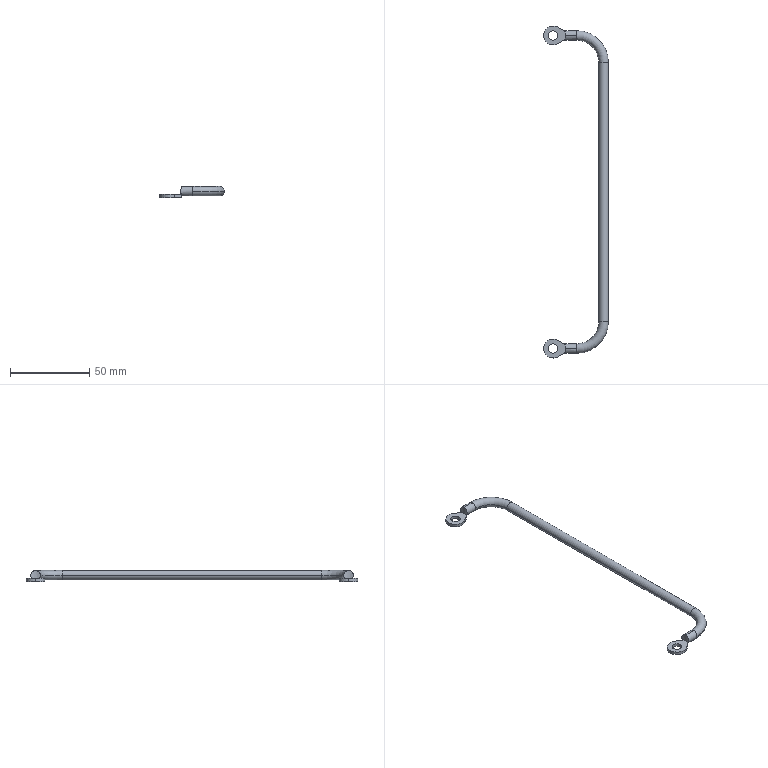Part | SolidWorks | features BaseBody 1 | 1 solid | 30 faces | box 41 x 210 x 7 mm | volume 6943 mm3 | cylinder 16 | plane 10 | torus 4 | commonest cylinder face diameters 6 x10 12 x4 16 x2
STEP:
#1=CARTESIAN_POINT('',(7.681,2.236,-4.));
#2=VERTEX_POINT('',#1);
#3=CARTESIAN_POINT('',(7.681,2.236,-2.));
#4=VERTEX_POINT('',#3);
#5=CARTESIAN_POINT('',(7.681,2.236,-15.078));
#6=DIRECTION('',(0.,0.,1.));
#7=VECTOR('',#6,1000.);
#8=LINE('',#5,#7);
#9=EDGE_CURVE('',#2,#4,#8,.T.);
#10=ORIENTED_EDGE('',*,*,#9,.F.);
#11=CARTESIAN_POINT('',(3.211,5.068,-4.));
#12=VERTEX_POINT('',#11);
#13=CARTESIAN_POINT('',(3.211,5.068,-4.));
#14=DIRECTION('',(-0.8447,0.5352,0.));
#15=VECTOR('',#14,1000.);
#16=LINE('',#13,#15);
#17=EDGE_CURVE('',#2,#12,#16,.T.);
#18=ORIENTED_EDGE('',*,*,#17,.T.);
#19=CARTESIAN_POINT('',(3.211,5.068,-2.));
#20=VERTEX_POINT('',#19);
#21=CARTESIAN_POINT('',(3.211,5.068,-15.078));
#22=DIRECTION('',(0.,0.,1.));
#23=VECTOR('',#22,1000.);
#24=LINE('',#21,#23);
#25=EDGE_CURVE('',#12,#20,#24,.T.);
#26=ORIENTED_EDGE('',*,*,#25,.T.);
#27=CARTESIAN_POINT('',(3.211,5.068,-2.));
#28=DIRECTION('',(0.8447,-0.5352,0.));
#29=VECTOR('',#28,1000.);
#30=LINE('',#27,#29);
#31=EDGE_CURVE('',#20,#4,#30,.T.);
#32=ORIENTED_EDGE('',*,*,#31,.T.);
#33=EDGE_LOOP('',(#10,#18,#26,#32));
#34=FACE_OUTER_BOUND('',#33,.T.);
#35=CARTESIAN_POINT('',(3.211,5.068,-15.078));
#36=DIRECTION('',(-0.5352,-0.8447,0.));
#37=DIRECTION('',(-0.8447,0.5352,0.));
#38=AXIS2_PLACEMENT_3D('',#35,#36,#37);
#39=PLANE('',#38);
#40=ADVANCED_FACE('',(#34),#39,.F.);
#41=CARTESIAN_POINT('',(7.681,-2.236,-2.));
#42=VERTEX_POINT('',#41);
#43=CARTESIAN_POINT('',(7.681,0.,-3.));
#44=VERTEX_POINT('',#43);
#45=CARTESIAN_POINT('',(7.681,0.,0.));
#46=DIRECTION('',(1.,0.,0.));
#47=DIRECTION('',(0.,0.,1.));
#48=AXIS2_PLACEMENT_3D('',#45,#46,#47);
#49=CIRCLE('',#48,3.);
#50=EDGE_CURVE('',#42,#44,#49,.T.);
#51=ORIENTED_EDGE('',*,*,#50,.F.);
#52=CARTESIAN_POINT('',(7.681,-2.236,-4.));
#53=VERTEX_POINT('',#52);
#54=CARTESIAN_POINT('',(7.681,-2.236,-15.078));
#55=DIRECTION('',(0.,0.,1.));
#56=VECTOR('',#55,1000.);
#57=LINE('',#54,#56);
#58=EDGE_CURVE('',#53,#42,#57,.T.);
#59=ORIENTED_EDGE('',*,*,#58,.F.);
#60=CARTESIAN_POINT('',(7.681,2.236,-4.));
#61=DIRECTION('',(0.,1.,0.));
#62=VECTOR('',#61,1000.);
#63=LINE('',#60,#62);
#64=EDGE_CURVE('',#53,#2,#63,.T.);
#65=ORIENTED_EDGE('',*,*,#64,.T.);
#66=ORIENTED_EDGE('',*,*,#9,.T.);
#67=CARTESIAN_POINT('',(7.681,0.,0.));
#68=DIRECTION('',(1.,0.,0.));
#69=DIRECTION('',(0.,0.,1.));
#70=AXIS2_PLACEMENT_3D('',#67,#68,#69);
#71=CIRCLE('',#70,3.);
#72=EDGE_CURVE('',#44,#4,#71,.T.);
#73=ORIENTED_EDGE('',*,*,#72,.F.);
#74=EDGE_LOOP('',(#51,#59,#65,#66,#73));
#75=FACE_OUTER_BOUND('',#74,.T.);
#76=CARTESIAN_POINT('',(7.681,2.236,-15.078));
#77=DIRECTION('',(-1.,0.,0.));
#78=DIRECTION('',(0.,0.,1.));
#79=AXIS2_PLACEMENT_3D('',#76,#77,#78);
#80=PLANE('',#79);
#81=ADVANCED_FACE('',(#75),#80,.F.);
#82=CARTESIAN_POINT('',(3.211,-5.068,-4.));
#83=VERTEX_POINT('',#82);
#84=CARTESIAN_POINT('',(3.211,-5.068,-2.));
#85=VERTEX_POINT('',#84);
#86=CARTESIAN_POINT('',(3.211,-5.068,-15.078));
#87=DIRECTION('',(0.,0.,1.));
#88=VECTOR('',#87,1000.);
#89=LINE('',#86,#88);
#90=EDGE_CURVE('',#83,#85,#89,.T.);
#91=ORIENTED_EDGE('',*,*,#90,.F.);
#92=CARTESIAN_POINT('',(7.681,-2.236,-4.));
#93=DIRECTION('',(0.8447,0.5352,0.));
#94=VECTOR('',#93,1000.);
#95=LINE('',#92,#94);
#96=EDGE_CURVE('',#83,#53,#95,.T.);
#97=ORIENTED_EDGE('',*,*,#96,.T.);
#98=ORIENTED_EDGE('',*,*,#58,.T.);
#99=CARTESIAN_POINT('',(7.681,-2.236,-2.));
#100=DIRECTION('',(-0.8447,-0.5352,0.));
#101=VECTOR('',#100,1000.);
#102=LINE('',#99,#101);
#103=EDGE_CURVE('',#42,#85,#102,.T.);
#104=ORIENTED_EDGE('',*,*,#103,.T.);
#105=EDGE_LOOP('',(#91,#97,#98,#104));
#106=FACE_OUTER_BOUND('',#105,.T.);
#107=CARTESIAN_POINT('',(7.681,-2.236,-15.078));
#108=DIRECTION('',(-0.5352,0.8447,0.));
#109=DIRECTION('',(0.,0.,1.));
#110=AXIS2_PLACEMENT_3D('',#107,#108,#109);
#111=PLANE('',#110);
#112=ADVANCED_FACE('',(#106),#111,.F.);
#113=CARTESIAN_POINT('',(7.681,200.236,-4.));
#114=VERTEX_POINT('',#113);
#115=CARTESIAN_POINT('',(7.681,200.236,-2.));
#116=VERTEX_POINT('',#115);
#117=CARTESIAN_POINT('',(7.681,200.236,-15.078));
#118=DIRECTION('',(0.,0.,1.));
#119=VECTOR('',#118,1000.);
#120=LINE('',#117,#119);
#121=EDGE_CURVE('',#114,#116,#120,.T.);
#122=ORIENTED_EDGE('',*,*,#121,.F.);
#123=CARTESIAN_POINT('',(3.211,203.068,-4.));
#124=VERTEX_POINT('',#123);
#125=CARTESIAN_POINT('',(3.211,203.068,-4.));
#126=DIRECTION('',(-0.8447,0.5352,0.));
#127=VECTOR('',#126,1000.);
#128=LINE('',#125,#127);
#129=EDGE_CURVE('',#114,#124,#128,.T.);
#130=ORIENTED_EDGE('',*,*,#129,.T.);
#131=CARTESIAN_POINT('',(3.211,203.068,-2.));
#132=VERTEX_POINT('',#131);
#133=CARTESIAN_POINT('',(3.211,203.068,-15.078));
#134=DIRECTION('',(0.,0.,1.));
#135=VECTOR('',#134,1000.);
#136=LINE('',#133,#135);
#137=EDGE_CURVE('',#124,#132,#136,.T.);
#138=ORIENTED_EDGE('',*,*,#137,.T.);
#139=CARTESIAN_POINT('',(3.211,203.068,-2.));
#140=DIRECTION('',(0.8447,-0.5352,0.));
#141=VECTOR('',#140,1000.);
#142=LINE('',#139,#141);
#143=EDGE_CURVE('',#132,#116,#142,.T.);
#144=ORIENTED_EDGE('',*,*,#143,.T.);
#145=EDGE_LOOP('',(#122,#130,#138,#144));
#146=FACE_OUTER_BOUND('',#145,.T.);
#147=CARTESIAN_POINT('',(3.211,203.068,-15.078));
#148=DIRECTION('',(-0.5352,-0.8447,0.));
#149=DIRECTION('',(-0.8447,0.5352,0.));
#150=AXIS2_PLACEMENT_3D('',#147,#148,#149);
#151=PLANE('',#150);
#152=ADVANCED_FACE('',(#146),#151,.F.);
#153=CARTESIAN_POINT('',(7.681,195.764,-2.));
#154=VERTEX_POINT('',#153);
#155=CARTESIAN_POINT('',(7.681,198.,-3.));
#156=VERTEX_POINT('',#155);
#157=CARTESIAN_POINT('',(7.681,198.,0.));
#158=DIRECTION('',(1.,0.,0.));
#159=DIRECTION('',(0.,-1.,0.));
#160=AXIS2_PLACEMENT_3D('',#157,#158,#159);
#161=CIRCLE('',#160,3.);
#162=EDGE_CURVE('',#154,#156,#161,.T.);
#163=ORIENTED_EDGE('',*,*,#162,.F.);
#164=CARTESIAN_POINT('',(7.681,195.764,-4.));
#165=VERTEX_POINT('',#164);
#166=CARTESIAN_POINT('',(7.681,195.764,-15.078));
#167=DIRECTION('',(0.,0.,1.));
#168=VECTOR('',#167,1000.);
#169=LINE('',#166,#168);
#170=EDGE_CURVE('',#165,#154,#169,.T.);
#171=ORIENTED_EDGE('',*,*,#170,.F.);
#172=CARTESIAN_POINT('',(7.681,200.236,-4.));
#173=DIRECTION('',(0.,1.,0.));
#174=VECTOR('',#173,1000.);
#175=LINE('',#172,#174);
#176=EDGE_CURVE('',#165,#114,#175,.T.);
#177=ORIENTED_EDGE('',*,*,#176,.T.);
#178=ORIENTED_EDGE('',*,*,#121,.T.);
#179=CARTESIAN_POINT('',(7.681,198.,0.));
#180=DIRECTION('',(1.,0.,0.));
#181=DIRECTION('',(0.,-1.,0.));
#182=AXIS2_PLACEMENT_3D('',#179,#180,#181);
#183=CIRCLE('',#182,3.);
#184=EDGE_CURVE('',#156,#116,#183,.T.);
#185=ORIENTED_EDGE('',*,*,#184,.F.);
#186=EDGE_LOOP('',(#163,#171,#177,#178,#185));
#187=FACE_OUTER_BOUND('',#186,.T.);
#188=CARTESIAN_POINT('',(7.681,200.236,-15.078));
#189=DIRECTION('',(-1.,0.,0.));
#190=DIRECTION('',(0.,0.,1.));
#191=AXIS2_PLACEMENT_3D('',#188,#189,#190);
#192=PLANE('',#191);
#193=ADVANCED_FACE('',(#187),#192,.F.);
#194=CARTESIAN_POINT('',(3.211,192.932,-4.));
#195=VERTEX_POINT('',#194);
#196=CARTESIAN_POINT('',(3.211,192.932,-2.));
#197=VERTEX_POINT('',#196);
#198=CARTESIAN_POINT('',(3.211,192.932,-15.078));
#199=DIRECTION('',(0.,0.,1.));
#200=VECTOR('',#199,1000.);
#201=LINE('',#198,#200);
#202=EDGE_CURVE('',#195,#197,#201,.T.);
#203=ORIENTED_EDGE('',*,*,#202,.F.);
#204=CARTESIAN_POINT('',(3.211,192.932,-4.));
#205=DIRECTION('',(0.8447,0.5352,0.));
#206=VECTOR('',#205,1000.);
#207=LINE('',#204,#206);
#208=EDGE_CURVE('',#195,#165,#207,.T.);
#209=ORIENTED_EDGE('',*,*,#208,.T.);
#210=ORIENTED_EDGE('',*,*,#170,.T.);
#211=CARTESIAN_POINT('',(3.211,192.932,-2.));
#212=DIRECTION('',(-0.8447,-0.5352,0.));
#213=VECTOR('',#212,1000.);
#214=LINE('',#211,#213);
#215=EDGE_CURVE('',#154,#197,#214,.T.);
#216=ORIENTED_EDGE('',*,*,#215,.T.);
#217=EDGE_LOOP('',(#203,#209,#210,#216));
#218=FACE_OUTER_BOUND('',#217,.T.);
#219=CARTESIAN_POINT('',(3.211,192.932,-15.078));
#220=DIRECTION('',(-0.5352,0.8447,0.));
#221=DIRECTION('',(0.,0.,1.));
#222=AXIS2_PLACEMENT_3D('',#219,#220,#221);
#223=PLANE('',#222);
#224=ADVANCED_FACE('',(#218),#223,.F.);
#225=CARTESIAN_POINT('',(0.,0.,-2.));
#226=DIRECTION('',(0.,0.,1.));
#227=DIRECTION('',(1.,0.,0.));
#228=AXIS2_PLACEMENT_3D('',#225,#226,#227);
#229=CIRCLE('',#228,8.);
#230=EDGE_CURVE('',#42,#4,#229,.T.);
#231=ORIENTED_EDGE('',*,*,#230,.F.);
#232=CARTESIAN_POINT('',(8.,0.,3.));
#233=VERTEX_POINT('',#232);
#234=CARTESIAN_POINT('',(8.,0.,3.));
#235=CARTESIAN_POINT('',(8.,-0.1411,3.));
#236=CARTESIAN_POINT('',(7.996,-0.284,2.99));
#237=CARTESIAN_POINT('',(7.985,-0.499,2.959));
#238=CARTESIAN_POINT('',(7.98,-0.5708,2.946));
#239=CARTESIAN_POINT('',(7.971,-0.6783,2.923));
#240=CARTESIAN_POINT('',(7.967,-0.732,2.91));
#241=CARTESIAN_POINT('',(7.96,-0.7945,2.893));
#242=CARTESIAN_POINT('',(7.958,-0.8212,2.885));
#243=CARTESIAN_POINT('',(7.956,-0.839,2.88));
#244=CARTESIAN_POINT('',(7.955,-0.8491,2.877));
#245=CARTESIAN_POINT('',(7.941,-0.9804,2.838));
#246=CARTESIAN_POINT('',(7.924,-1.109,2.791));
#247=CARTESIAN_POINT('',(7.893,-1.305,2.702));
#248=CARTESIAN_POINT('',(7.882,-1.371,2.669));
#249=CARTESIAN_POINT('',(7.864,-1.47,2.615));
#250=CARTESIAN_POINT('',(7.854,-1.52,2.587));
#251=CARTESIAN_POINT('',(7.843,-1.578,2.551));
#252=CARTESIAN_POINT('',(7.837,-1.607,2.533));
#253=CARTESIAN_POINT('',(7.834,-1.62,2.525));
#254=CARTESIAN_POINT('',(7.833,-1.628,2.52));
#255=CARTESIAN_POINT('',(7.832,-1.633,2.516));
#256=CARTESIAN_POINT('',(7.82,-1.687,2.481));
#257=CARTESIAN_POINT('',(7.808,-1.741,2.444));
#258=CARTESIAN_POINT('',(7.789,-1.827,2.38));
#259=CARTESIAN_POINT('',(7.782,-1.856,2.357));
#260=CARTESIAN_POINT('',(7.771,-1.901,2.321));
#261=CARTESIAN_POINT('',(7.765,-1.924,2.302));
#262=CARTESIAN_POINT('',(7.76,-1.947,2.283));
#263=CARTESIAN_POINT('',(7.756,-1.962,2.27));
#264=CARTESIAN_POINT('',(7.753,-1.971,2.262));
#265=CARTESIAN_POINT('',(7.738,-2.031,2.209));
#266=CARTESIAN_POINT('',(7.717,-2.109,2.136));
#267=CARTESIAN_POINT('',(7.693,-2.195,2.046));
#268=CARTESIAN_POINT('',(7.681,-2.237,1.999));
#269=CARTESIAN_POINT('',(7.676,-2.254,1.979));
#270=CARTESIAN_POINT('',(7.672,-2.266,1.966));
#271=CARTESIAN_POINT('',(7.671,-2.271,1.96));
#272=CARTESIAN_POINT('',(7.636,-2.386,1.826));
#273=CARTESIAN_POINT('',(7.608,-2.476,1.7));
#274=CARTESIAN_POINT('',(7.57,-2.589,1.518));
#275=CARTESIAN_POINT('',(7.558,-2.622,1.459));
#276=CARTESIAN_POINT('',(7.542,-2.668,1.371));
#277=CARTESIAN_POINT('',(7.534,-2.69,1.329));
#278=CARTESIAN_POINT('',(7.526,-2.713,1.28));
#279=CARTESIAN_POINT('',(7.522,-2.723,1.259));
#280=CARTESIAN_POINT('',(7.52,-2.729,1.245));
#281=CARTESIAN_POINT('',(7.519,-2.732,1.24));
#282=CARTESIAN_POINT('',(7.495,-2.799,1.091));
#283=CARTESIAN_POINT('',(7.476,-2.849,0.9501));
#284=CARTESIAN_POINT('',(7.453,-2.908,0.7416));
#285=CARTESIAN_POINT('',(7.446,-2.924,0.6726));
#286=CARTESIAN_POINT('',(7.438,-2.946,0.5701));
#287=CARTESIAN_POINT('',(7.434,-2.955,0.5191));
#288=CARTESIAN_POINT('',(7.431,-2.963,0.4685));
#289=CARTESIAN_POINT('',(7.429,-2.968,0.435));
#290=CARTESIAN_POINT('',(7.428,-2.971,0.4194));
#291=CARTESIAN_POINT('',(7.419,-2.992,0.2582));
#292=CARTESIAN_POINT('',(7.416,-3.001,0.1133));
#293=CARTESIAN_POINT('',(7.417,-2.999,-0.1042));
#294=CARTESIAN_POINT('',(7.418,-2.996,-0.1767));
#295=CARTESIAN_POINT('',(7.422,-2.987,-0.2852));
#296=CARTESIAN_POINT('',(7.424,-2.981,-0.3393));
#297=CARTESIAN_POINT('',(7.427,-2.974,-0.3934));
#298=CARTESIAN_POINT('',(7.429,-2.969,-0.4293));
#299=CARTESIAN_POINT('',(7.43,-2.966,-0.4488));
#300=CARTESIAN_POINT('',(7.439,-2.943,-0.5972));
#301=CARTESIAN_POINT('',(7.451,-2.913,-0.733));
#302=CARTESIAN_POINT('',(7.475,-2.85,-0.94));
#303=CARTESIAN_POINT('',(7.484,-2.826,-1.009));
#304=CARTESIAN_POINT('',(7.499,-2.786,-1.114));
#305=CARTESIAN_POINT('',(7.507,-2.764,-1.166));
#306=CARTESIAN_POINT('',(7.517,-2.737,-1.228));
#307=CARTESIAN_POINT('',(7.522,-2.723,-1.258));
#308=CARTESIAN_POINT('',(7.524,-2.717,-1.271));
#309=CARTESIAN_POINT('',(7.526,-2.713,-1.28));
#310=CARTESIAN_POINT('',(7.527,-2.71,-1.286));
#311=CARTESIAN_POINT('',(7.56,-2.618,-1.48));
#312=CARTESIAN_POINT('',(7.611,-2.476,-1.732));
#313=CARTESIAN_POINT('',(7.681,-2.236,-2.));
#314=B_SPLINE_CURVE_WITH_KNOTS('',3,(#234,#235,#236,#237,#238,#239,#240,#241,#242,#243,#244,#245,#246,#247,#248,#249,#250,#251,#252,#253,#254,#255,#256,#257,#258,#259,#260,#261,#262,#263,#264,#265,#266,#267,#268,#269,#270,#271,#272,#273,#274,#275,#276,#277,#278,#279,#280,#281,#282,#283,#284,#285,#286,#287,#288,#289,#290,#291,#292,#293,#294,#295,#296,#297,#298,#299,#300,#301,#302,#303,#304,#305,#306,#307,#308,#309,#310,#311,#312,#313),.UNSPECIFIED.,.F.,.F.,(4,2,2,1,1,2,2,2,2,1,1,1,2,2,2,2,1,2,2,1,1,1,2,2,2,2,1,1,2,2,2,2,1,2,2,2,2,1,2,2,2,2,1,1,1,2,2,4),(0.,0.0625,0.09375,0.1094,0.1172,0.1211,0.125,0.1875,0.2187,0.2344,0.2422,0.2461,0.248,0.25,0.2812,0.2969,0.3047,0.3086,0.3125,0.3437,0.3594,0.3672,0.3711,0.375,0.4375,0.4687,0.4844,0.4922,0.4961,0.5,0.5625,0.5937,0.6094,0.6172,0.625,0.6875,0.7187,0.7344,0.7422,0.75,0.8125,0.8437,0.8594,0.8672,0.8711,0.873,0.875,1.),.UNSPECIFIED.);
#315=EDGE_CURVE('',#233,#42,#314,.T.);
#316=ORIENTED_EDGE('',*,*,#315,.F.);
#317=CARTESIAN_POINT('',(7.681,2.236,-2.));
#318=CARTESIAN_POINT('',(7.646,2.356,-1.866));
#319=CARTESIAN_POINT('',(7.616,2.452,-1.735));
#320=CARTESIAN_POINT('',(7.577,2.567,-1.554));
#321=CARTESIAN_POINT('',(7.566,2.601,-1.497));
#322=CARTESIAN_POINT('',(7.55,2.646,-1.415));
#323=CARTESIAN_POINT('',(7.543,2.667,-1.375));
#324=CARTESIAN_POINT('',(7.535,2.689,-1.331));
#325=CARTESIAN_POINT('',(7.531,2.699,-1.309));
#326=CARTESIAN_POINT('',(7.529,2.704,-1.3));
#327=CARTESIAN_POINT('',(7.528,2.706,-1.294));
#328=CARTESIAN_POINT('',(7.528,2.707,-1.293));
#329=CARTESIAN_POINT('',(7.503,2.776,-1.149));
#330=CARTESIAN_POINT('',(7.483,2.829,-1.009));
#331=CARTESIAN_POINT('',(7.459,2.892,-0.8019));
#332=CARTESIAN_POINT('',(7.452,2.91,-0.7335));
#333=CARTESIAN_POINT('',(7.443,2.933,-0.632));
#334=CARTESIAN_POINT('',(7.439,2.943,-0.5815));
#335=CARTESIAN_POINT('',(7.435,2.953,-0.5315));
#336=CARTESIAN_POINT('',(7.433,2.958,-0.4983));
#337=CARTESIAN_POINT('',(7.432,2.961,-0.4832));
#338=CARTESIAN_POINT('',(7.422,2.986,-0.3218));
#339=CARTESIAN_POINT('',(7.417,2.998,-0.1769));
#340=CARTESIAN_POINT('',(7.416,3.001,0.04039));
#341=CARTESIAN_POINT('',(7.417,2.999,0.1128));
#342=CARTESIAN_POINT('',(7.419,2.992,0.2211));
#343=CARTESIAN_POINT('',(7.421,2.988,0.2752));
#344=CARTESIAN_POINT('',(7.423,2.982,0.3292));
#345=CARTESIAN_POINT('',(7.425,2.978,0.3651));
#346=CARTESIAN_POINT('',(7.426,2.975,0.3842));
#347=CARTESIAN_POINT('',(7.434,2.955,0.5349));
#348=CARTESIAN_POINT('',(7.445,2.927,0.6725));
#349=CARTESIAN_POINT('',(7.468,2.868,0.8818));
#350=CARTESIAN_POINT('',(7.477,2.846,0.9521));
#351=CARTESIAN_POINT('',(7.491,2.808,1.058));
#352=CARTESIAN_POINT('',(7.499,2.787,1.111));
#353=CARTESIAN_POINT('',(7.508,2.762,1.172));
#354=CARTESIAN_POINT('',(7.513,2.748,1.203));
#355=CARTESIAN_POINT('',(7.515,2.742,1.217));
#356=CARTESIAN_POINT('',(7.517,2.738,1.225));
#357=CARTESIAN_POINT('',(7.518,2.736,1.231));
#358=CARTESIAN_POINT('',(7.535,2.689,1.334));
#359=CARTESIAN_POINT('',(7.555,2.632,1.447));
#360=CARTESIAN_POINT('',(7.593,2.52,1.63));
#361=CARTESIAN_POINT('',(7.607,2.478,1.693));
#362=CARTESIAN_POINT('',(7.629,2.408,1.79));
#363=CARTESIAN_POINT('',(7.641,2.371,1.838));
#364=CARTESIAN_POINT('',(7.655,2.325,1.896));
#365=CARTESIAN_POINT('',(7.661,2.304,1.921));
#366=CARTESIAN_POINT('',(7.665,2.29,1.938));
#367=CARTESIAN_POINT('',(7.668,2.282,1.948));
#368=CARTESIAN_POINT('',(7.697,2.183,2.062));
#369=CARTESIAN_POINT('',(7.725,2.082,2.164));
#370=CARTESIAN_POINT('',(7.766,1.923,2.304));
#371=CARTESIAN_POINT('',(7.779,1.868,2.349));
#372=CARTESIAN_POINT('',(7.799,1.782,2.413));
#373=CARTESIAN_POINT('',(7.809,1.739,2.445));
#374=CARTESIAN_POINT('',(7.818,1.695,2.475));
#375=CARTESIAN_POINT('',(7.825,1.665,2.495));
#376=CARTESIAN_POINT('',(7.828,1.652,2.504));
#377=CARTESIAN_POINT('',(7.859,1.503,2.601));
#378=CARTESIAN_POINT('',(7.883,1.37,2.673));
#379=CARTESIAN_POINT('',(7.914,1.174,2.762));
#380=CARTESIAN_POINT('',(7.923,1.109,2.788));
#381=CARTESIAN_POINT('',(7.936,1.013,2.824));
#382=CARTESIAN_POINT('',(7.942,0.9659,2.841));
#383=CARTESIAN_POINT('',(7.948,0.9112,2.858));
#384=CARTESIAN_POINT('',(7.951,0.8879,2.866));
#385=CARTESIAN_POINT('',(7.952,0.8724,2.87));
#386=CARTESIAN_POINT('',(7.953,0.8659,2.872));
#387=CARTESIAN_POINT('',(7.985,0.5721,2.96));
#388=CARTESIAN_POINT('',(8.,0.2822,3.));
#389=CARTESIAN_POINT('',(8.,0.,3.));
#390=B_SPLINE_CURVE_WITH_KNOTS('',3,(#317,#318,#319,#320,#321,#322,#323,#324,#325,#326,#327,#328,#329,#330,#331,#332,#333,#334,#335,#336,#337,#338,#339,#340,#341,#342,#343,#344,#345,#346,#347,#348,#349,#350,#351,#352,#353,#354,#355,#356,#357,#358,#359,#360,#361,#362,#363,#364,#365,#366,#367,#368,#369,#370,#371,#372,#373,#374,#375,#376,#377,#378,#379,#380,#381,#382,#383,#384,#385,#386,#387,#388,#389),.UNSPECIFIED.,.F.,.F.,(4,2,2,1,1,1,2,2,2,2,1,2,2,2,2,1,2,2,2,2,1,1,1,2,2,2,2,1,1,2,2,2,2,1,2,2,2,2,1,1,2,2,4),(0.,0.0625,0.09375,0.1094,0.1172,0.1211,0.123,0.125,0.1875,0.2188,0.2344,0.2422,0.25,0.3125,0.3438,0.3594,0.3672,0.375,0.4375,0.4688,0.4844,0.4922,0.4961,0.498,0.5,0.5625,0.5938,0.6094,0.6172,0.6211,0.625,0.6875,0.7188,0.7344,0.7422,0.75,0.8125,0.8438,0.8594,0.8672,0.8711,0.875,1.),.UNSPECIFIED.);
#391=EDGE_CURVE('',#4,#233,#390,.T.);
#392=ORIENTED_EDGE('',*,*,#391,.F.);
#393=EDGE_LOOP('',(#231,#316,#392));
#394=FACE_OUTER_BOUND('',#393,.T.);
#395=CARTESIAN_POINT('',(0.,0.,13.));
#396=DIRECTION('',(0.,0.,-1.));
#397=DIRECTION('',(-1.,0.,0.));
#398=AXIS2_PLACEMENT_3D('',#395,#396,#397);
#399=CYLINDRICAL_SURFACE('',#398,8.);
#400=ADVANCED_FACE('',(#394),#399,.F.);
#401=CARTESIAN_POINT('',(0.,198.,-2.));
#402=DIRECTION('',(0.,0.,1.));
#403=DIRECTION('',(1.,0.,0.));
#404=AXIS2_PLACEMENT_3D('',#401,#402,#403);
#405=CIRCLE('',#404,8.);
#406=EDGE_CURVE('',#154,#116,#405,.T.);
#407=ORIENTED_EDGE('',*,*,#406,.F.);
#408=CARTESIAN_POINT('',(8.,198.,3.));
#409=VERTEX_POINT('',#408);
#410=CARTESIAN_POINT('',(8.,198.,3.));
#411=CARTESIAN_POINT('',(8.,197.859,3.));
#412=CARTESIAN_POINT('',(7.996,197.716,2.99));
#413=CARTESIAN_POINT('',(7.985,197.501,2.959));
#414=CARTESIAN_POINT('',(7.98,197.429,2.946));
#415=CARTESIAN_POINT('',(7.971,197.322,2.923));
#416=CARTESIAN_POINT('',(7.967,197.268,2.91));
#417=CARTESIAN_POINT('',(7.96,197.206,2.893));
#418=CARTESIAN_POINT('',(7.958,197.179,2.885));
#419=CARTESIAN_POINT('',(7.956,197.161,2.88));
#420=CARTESIAN_POINT('',(7.955,197.151,2.877));
#421=CARTESIAN_POINT('',(7.941,197.02,2.838));
#422=CARTESIAN_POINT('',(7.924,196.891,2.791));
#423=CARTESIAN_POINT('',(7.893,196.695,2.702));
#424=CARTESIAN_POINT('',(7.882,196.629,2.669));
#425=CARTESIAN_POINT('',(7.864,196.53,2.615));
#426=CARTESIAN_POINT('',(7.854,196.48,2.587));
#427=CARTESIAN_POINT('',(7.843,196.422,2.551));
#428=CARTESIAN_POINT('',(7.837,196.393,2.533));
#429=CARTESIAN_POINT('',(7.834,196.38,2.525));
#430=CARTESIAN_POINT('',(7.833,196.372,2.52));
#431=CARTESIAN_POINT('',(7.832,196.367,2.516));
#432=CARTESIAN_POINT('',(7.82,196.313,2.481));
#433=CARTESIAN_POINT('',(7.808,196.259,2.444));
#434=CARTESIAN_POINT('',(7.789,196.173,2.38));
#435=CARTESIAN_POINT('',(7.782,196.144,2.357));
#436=CARTESIAN_POINT('',(7.771,196.099,2.321));
#437=CARTESIAN_POINT('',(7.765,196.076,2.302));
#438=CARTESIAN_POINT('',(7.76,196.053,2.283));
#439=CARTESIAN_POINT('',(7.756,196.038,2.27));
#440=CARTESIAN_POINT('',(7.753,196.029,2.262));
#441=CARTESIAN_POINT('',(7.738,195.969,2.209));
#442=CARTESIAN_POINT('',(7.717,195.891,2.136));
#443=CARTESIAN_POINT('',(7.693,195.805,2.046));
#444=CARTESIAN_POINT('',(7.681,195.763,1.999));
#445=CARTESIAN_POINT('',(7.676,195.746,1.979));
#446=CARTESIAN_POINT('',(7.672,195.734,1.966));
#447=CARTESIAN_POINT('',(7.671,195.729,1.96));
#448=CARTESIAN_POINT('',(7.636,195.614,1.826));
#449=CARTESIAN_POINT('',(7.608,195.524,1.7));
#450=CARTESIAN_POINT('',(7.57,195.411,1.518));
#451=CARTESIAN_POINT('',(7.558,195.378,1.459));
#452=CARTESIAN_POINT('',(7.542,195.332,1.371));
#453=CARTESIAN_POINT('',(7.534,195.31,1.329));
#454=CARTESIAN_POINT('',(7.526,195.287,1.28));
#455=CARTESIAN_POINT('',(7.522,195.277,1.259));
#456=CARTESIAN_POINT('',(7.52,195.271,1.245));
#457=CARTESIAN_POINT('',(7.519,195.268,1.24));
#458=CARTESIAN_POINT('',(7.495,195.201,1.091));
#459=CARTESIAN_POINT('',(7.476,195.151,0.9501));
#460=CARTESIAN_POINT('',(7.453,195.092,0.7416));
#461=CARTESIAN_POINT('',(7.446,195.076,0.6726));
#462=CARTESIAN_POINT('',(7.438,195.054,0.5701));
#463=CARTESIAN_POINT('',(7.434,195.045,0.5191));
#464=CARTESIAN_POINT('',(7.431,195.037,0.4685));
#465=CARTESIAN_POINT('',(7.429,195.032,0.435));
#466=CARTESIAN_POINT('',(7.428,195.029,0.4194));
#467=CARTESIAN_POINT('',(7.419,195.008,0.2582));
#468=CARTESIAN_POINT('',(7.416,194.999,0.1133));
#469=CARTESIAN_POINT('',(7.417,195.001,-0.1042));
#470=CARTESIAN_POINT('',(7.418,195.004,-0.1767));
#471=CARTESIAN_POINT('',(7.422,195.013,-0.2852));
#472=CARTESIAN_POINT('',(7.424,195.019,-0.3393));
#473=CARTESIAN_POINT('',(7.427,195.026,-0.3934));
#474=CARTESIAN_POINT('',(7.429,195.031,-0.4293));
#475=CARTESIAN_POINT('',(7.43,195.034,-0.4488));
#476=CARTESIAN_POINT('',(7.439,195.057,-0.5972));
#477=CARTESIAN_POINT('',(7.451,195.087,-0.733));
#478=CARTESIAN_POINT('',(7.475,195.15,-0.94));
#479=CARTESIAN_POINT('',(7.484,195.174,-1.009));
#480=CARTESIAN_POINT('',(7.499,195.214,-1.114));
#481=CARTESIAN_POINT('',(7.507,195.236,-1.166));
#482=CARTESIAN_POINT('',(7.517,195.263,-1.228));
#483=CARTESIAN_POINT('',(7.522,195.277,-1.258));
#484=CARTESIAN_POINT('',(7.524,195.283,-1.271));
#485=CARTESIAN_POINT('',(7.526,195.287,-1.28));
#486=CARTESIAN_POINT('',(7.527,195.29,-1.286));
#487=CARTESIAN_POINT('',(7.56,195.382,-1.48));
#488=CARTESIAN_POINT('',(7.611,195.524,-1.732));
#489=CARTESIAN_POINT('',(7.681,195.764,-2.));
#490=B_SPLINE_CURVE_WITH_KNOTS('',3,(#410,#411,#412,#413,#414,#415,#416,#417,#418,#419,#420,#421,#422,#423,#424,#425,#426,#427,#428,#429,#430,#431,#432,#433,#434,#435,#436,#437,#438,#439,#440,#441,#442,#443,#444,#445,#446,#447,#448,#449,#450,#451,#452,#453,#454,#455,#456,#457,#458,#459,#460,#461,#462,#463,#464,#465,#466,#467,#468,#469,#470,#471,#472,#473,#474,#475,#476,#477,#478,#479,#480,#481,#482,#483,#484,#485,#486,#487,#488,#489),.UNSPECIFIED.,.F.,.F.,(4,2,2,1,1,2,2,2,2,1,1,1,2,2,2,2,1,2,2,1,1,1,2,2,2,2,1,1,2,2,2,2,1,2,2,2,2,1,2,2,2,2,1,1,1,2,2,4),(0.,0.0625,0.09375,0.1094,0.1172,0.1211,0.125,0.1875,0.2187,0.2344,0.2422,0.2461,0.248,0.25,0.2812,0.2969,0.3047,0.3086,0.3125,0.3437,0.3594,0.3672,0.3711,0.375,0.4375,0.4687,0.4844,0.4922,0.4961,0.5,0.5625,0.5937,0.6094,0.6172,0.625,0.6875,0.7187,0.7344,0.7422,0.75,0.8125,0.8437,0.8594,0.8672,0.8711,0.873,0.875,1.),.UNSPECIFIED.);
#491=EDGE_CURVE('',#409,#154,#490,.T.);
#492=ORIENTED_EDGE('',*,*,#491,.F.);
#493=CARTESIAN_POINT('',(7.681,200.236,-2.));
#494=CARTESIAN_POINT('',(7.646,200.356,-1.866));
#495=CARTESIAN_POINT('',(7.616,200.452,-1.735));
#496=CARTESIAN_POINT('',(7.577,200.567,-1.554));
#497=CARTESIAN_POINT('',(7.566,200.601,-1.497));
#498=CARTESIAN_POINT('',(7.55,200.646,-1.415));
#499=CARTESIAN_POINT('',(7.543,200.667,-1.375));
#500=CARTESIAN_POINT('',(7.535,200.689,-1.331));
#501=CARTESIAN_POINT('',(7.531,200.699,-1.309));
#502=CARTESIAN_POINT('',(7.529,200.704,-1.3));
#503=CARTESIAN_POINT('',(7.528,200.706,-1.294));
#504=CARTESIAN_POINT('',(7.528,200.707,-1.293));
#505=CARTESIAN_POINT('',(7.503,200.776,-1.149));
#506=CARTESIAN_POINT('',(7.483,200.829,-1.009));
#507=CARTESIAN_POINT('',(7.459,200.892,-0.8019));
#508=CARTESIAN_POINT('',(7.452,200.91,-0.7335));
#509=CARTESIAN_POINT('',(7.443,200.933,-0.632));
#510=CARTESIAN_POINT('',(7.439,200.943,-0.5815));
#511=CARTESIAN_POINT('',(7.435,200.953,-0.5315));
#512=CARTESIAN_POINT('',(7.433,200.958,-0.4983));
#513=CARTESIAN_POINT('',(7.432,200.961,-0.4832));
#514=CARTESIAN_POINT('',(7.422,200.986,-0.3218));
#515=CARTESIAN_POINT('',(7.417,200.998,-0.1769));
#516=CARTESIAN_POINT('',(7.416,201.001,0.04039));
#517=CARTESIAN_POINT('',(7.417,200.999,0.1128));
#518=CARTESIAN_POINT('',(7.419,200.992,0.2211));
#519=CARTESIAN_POINT('',(7.421,200.988,0.2752));
#520=CARTESIAN_POINT('',(7.423,200.982,0.3292));
#521=CARTESIAN_POINT('',(7.425,200.978,0.3651));
#522=CARTESIAN_POINT('',(7.426,200.975,0.3842));
#523=CARTESIAN_POINT('',(7.434,200.955,0.5349));
#524=CARTESIAN_POINT('',(7.445,200.927,0.6725));
#525=CARTESIAN_POINT('',(7.468,200.868,0.8818));
#526=CARTESIAN_POINT('',(7.477,200.846,0.9521));
#527=CARTESIAN_POINT('',(7.491,200.808,1.058));
#528=CARTESIAN_POINT('',(7.499,200.787,1.111));
#529=CARTESIAN_POINT('',(7.508,200.762,1.172));
#530=CARTESIAN_POINT('',(7.513,200.748,1.203));
#531=CARTESIAN_POINT('',(7.515,200.742,1.217));
#532=CARTESIAN_POINT('',(7.517,200.738,1.225));
#533=CARTESIAN_POINT('',(7.518,200.736,1.231));
#534=CARTESIAN_POINT('',(7.535,200.689,1.334));
#535=CARTESIAN_POINT('',(7.555,200.632,1.447));
#536=CARTESIAN_POINT('',(7.593,200.52,1.63));
#537=CARTESIAN_POINT('',(7.607,200.478,1.693));
#538=CARTESIAN_POINT('',(7.629,200.408,1.79));
#539=CARTESIAN_POINT('',(7.641,200.371,1.838));
#540=CARTESIAN_POINT('',(7.655,200.325,1.896));
#541=CARTESIAN_POINT('',(7.661,200.304,1.921));
#542=CARTESIAN_POINT('',(7.665,200.29,1.938));
#543=CARTESIAN_POINT('',(7.668,200.282,1.948));
#544=CARTESIAN_POINT('',(7.697,200.183,2.062));
#545=CARTESIAN_POINT('',(7.725,200.082,2.164));
#546=CARTESIAN_POINT('',(7.766,199.923,2.304));
#547=CARTESIAN_POINT('',(7.779,199.868,2.349));
#548=CARTESIAN_POINT('',(7.799,199.782,2.413));
#549=CARTESIAN_POINT('',(7.809,199.739,2.445));
#550=CARTESIAN_POINT('',(7.818,199.695,2.475));
#551=CARTESIAN_POINT('',(7.825,199.665,2.495));
#552=CARTESIAN_POINT('',(7.828,199.652,2.504));
#553=CARTESIAN_POINT('',(7.859,199.503,2.601));
#554=CARTESIAN_POINT('',(7.883,199.37,2.673));
#555=CARTESIAN_POINT('',(7.914,199.174,2.762));
#556=CARTESIAN_POINT('',(7.923,199.109,2.788));
#557=CARTESIAN_POINT('',(7.936,199.013,2.824));
#558=CARTESIAN_POINT('',(7.942,198.966,2.841));
#559=CARTESIAN_POINT('',(7.948,198.911,2.858));
#560=CARTESIAN_POINT('',(7.951,198.888,2.866));
#561=CARTESIAN_POINT('',(7.952,198.872,2.87));
#562=CARTESIAN_POINT('',(7.953,198.866,2.872));
#563=CARTESIAN_POINT('',(7.985,198.572,2.96));
#564=CARTESIAN_POINT('',(8.,198.282,3.));
#565=CARTESIAN_POINT('',(8.,198.,3.));
#566=B_SPLINE_CURVE_WITH_KNOTS('',3,(#493,#494,#495,#496,#497,#498,#499,#500,#501,#502,#503,#504,#505,#506,#507,#508,#509,#510,#511,#512,#513,#514,#515,#516,#517,#518,#519,#520,#521,#522,#523,#524,#525,#526,#527,#528,#529,#530,#531,#532,#533,#534,#535,#536,#537,#538,#539,#540,#541,#542,#543,#544,#545,#546,#547,#548,#549,#550,#551,#552,#553,#554,#555,#556,#557,#558,#559,#560,#561,#562,#563,#564,#565),.UNSPECIFIED.,.F.,.F.,(4,2,2,1,1,1,2,2,2,2,1,2,2,2,2,1,2,2,2,2,1,1,1,2,2,2,2,1,1,2,2,2,2,1,2,2,2,2,1,1,2,2,4),(0.,0.0625,0.09375,0.1094,0.1172,0.1211,0.123,0.125,0.1875,0.2188,0.2344,0.2422,0.25,0.3125,0.3438,0.3594,0.3672,0.375,0.4375,0.4688,0.4844,0.4922,0.4961,0.498,0.5,0.5625,0.5938,0.6094,0.6172,0.6211,0.625,0.6875,0.7188,0.7344,0.7422,0.75,0.8125,0.8438,0.8594,0.8672,0.8711,0.875,1.),.UNSPECIFIED.);
#567=EDGE_CURVE('',#116,#409,#566,.T.);
#568=ORIENTED_EDGE('',*,*,#567,.F.);
#569=EDGE_LOOP('',(#407,#492,#568));
#570=FACE_OUTER_BOUND('',#569,.T.);
#571=CARTESIAN_POINT('',(0.,198.,13.));
#572=DIRECTION('',(0.,0.,-1.));
#573=DIRECTION('',(-1.,0.,0.));
#574=AXIS2_PLACEMENT_3D('',#571,#572,#573);
#575=CYLINDRICAL_SURFACE('',#574,8.);
#576=ADVANCED_FACE('',(#570),#575,.F.);
#577=CARTESIAN_POINT('',(3.,198.,-2.));
#578=VERTEX_POINT('',#577);
#579=CARTESIAN_POINT('',(3.,198.,-4.));
#580=VERTEX_POINT('',#579);
#581=CARTESIAN_POINT('',(3.,198.,1.));
#582=DIRECTION('',(0.,0.,-1.));
#583=VECTOR('',#582,1000.);
#584=LINE('',#581,#583);
#585=EDGE_CURVE('',#578,#580,#584,.T.);
#586=ORIENTED_EDGE('',*,*,#585,.F.);
#587=CARTESIAN_POINT('',(-3.,198.,-2.));
#588=VERTEX_POINT('',#587);
#589=CARTESIAN_POINT('',(0.,198.,-2.));
#590=DIRECTION('',(0.,0.,1.));
#591=DIRECTION('',(1.,0.,0.));
#592=AXIS2_PLACEMENT_3D('',#589,#590,#591);
#593=CIRCLE('',#592,3.);
#594=EDGE_CURVE('',#578,#588,#593,.T.);
#595=ORIENTED_EDGE('',*,*,#594,.T.);
#596=CARTESIAN_POINT('',(-3.,198.,-4.));
#597=VERTEX_POINT('',#596);
#598=CARTESIAN_POINT('',(-3.,198.,1.));
#599=DIRECTION('',(0.,0.,-1.));
#600=VECTOR('',#599,1000.);
#601=LINE('',#598,#600);
#602=EDGE_CURVE('',#588,#597,#601,.T.);
#603=ORIENTED_EDGE('',*,*,#602,.T.);
#604=CARTESIAN_POINT('',(0.,198.,-4.));
#605=DIRECTION('',(0.,0.,1.));
#606=DIRECTION('',(1.,0.,0.));
#607=AXIS2_PLACEMENT_3D('',#604,#605,#606);
#608=CIRCLE('',#607,3.);
#609=EDGE_CURVE('',#580,#597,#608,.T.);
#610=ORIENTED_EDGE('',*,*,#609,.F.);
#611=EDGE_LOOP('',(#586,#595,#603,#610));
#612=FACE_OUTER_BOUND('',#611,.T.);
#613=CARTESIAN_POINT('',(0.,198.,1.));
#614=DIRECTION('',(0.,0.,-1.));
#615=DIRECTION('',(-1.,0.,0.));
#616=AXIS2_PLACEMENT_3D('',#613,#614,#615);
#617=CYLINDRICAL_SURFACE('',#616,3.);
#618=ADVANCED_FACE('',(#612),#617,.F.);
#619=CARTESIAN_POINT('',(0.,198.,-4.));
#620=DIRECTION('',(0.,0.,1.));
#621=DIRECTION('',(1.,0.,0.));
#622=AXIS2_PLACEMENT_3D('',#619,#620,#621);
#623=CIRCLE('',#622,3.);
#624=EDGE_CURVE('',#597,#580,#623,.T.);
#625=ORIENTED_EDGE('',*,*,#624,.T.);
#626=ORIENTED_EDGE('',*,*,#609,.T.);
#627=EDGE_LOOP('',(#625,#626));
#628=FACE_BOUND('',#627,.T.);
#629=CARTESIAN_POINT('',(-6.,198.,-4.));
#630=VERTEX_POINT('',#629);
#631=CARTESIAN_POINT('',(0.,198.,-4.));
#632=DIRECTION('',(0.,0.,1.));
#633=DIRECTION('',(1.,0.,0.));
#634=AXIS2_PLACEMENT_3D('',#631,#632,#633);
#635=CIRCLE('',#634,6.);
#636=EDGE_CURVE('',#124,#630,#635,.T.);
#637=ORIENTED_EDGE('',*,*,#636,.F.);
#638=ORIENTED_EDGE('',*,*,#129,.F.);
#639=ORIENTED_EDGE('',*,*,#176,.F.);
#640=ORIENTED_EDGE('',*,*,#208,.F.);
#641=CARTESIAN_POINT('',(0.,198.,-4.));
#642=DIRECTION('',(0.,0.,1.));
#643=DIRECTION('',(1.,0.,0.));
#644=AXIS2_PLACEMENT_3D('',#641,#642,#643);
#645=CIRCLE('',#644,6.);
#646=EDGE_CURVE('',#630,#195,#645,.T.);
#647=ORIENTED_EDGE('',*,*,#646,.F.);
#648=EDGE_LOOP('',(#637,#638,#639,#640,#647));
#649=FACE_OUTER_BOUND('',#648,.T.);
#650=CARTESIAN_POINT('',(0.,198.,-4.));
#651=DIRECTION('',(0.,0.,1.));
#652=DIRECTION('',(1.,0.,0.));
#653=AXIS2_PLACEMENT_3D('',#650,#651,#652);
#654=PLANE('',#653);
#655=ADVANCED_FACE('',(#628,#649),#654,.F.);
#656=CARTESIAN_POINT('',(0.,198.,-2.));
#657=DIRECTION('',(0.,0.,1.));
#658=DIRECTION('',(1.,0.,0.));
#659=AXIS2_PLACEMENT_3D('',#656,#657,#658);
#660=CIRCLE('',#659,3.);
#661=EDGE_CURVE('',#588,#578,#660,.T.);
#662=ORIENTED_EDGE('',*,*,#661,.F.);
#663=ORIENTED_EDGE('',*,*,#594,.F.);
#664=EDGE_LOOP('',(#662,#663));
#665=FACE_BOUND('',#664,.T.);
#666=ORIENTED_EDGE('',*,*,#406,.T.);
#667=ORIENTED_EDGE('',*,*,#143,.F.);
#668=CARTESIAN_POINT('',(-6.,198.,-2.));
#669=VERTEX_POINT('',#668);
#670=CARTESIAN_POINT('',(0.,198.,-2.));
#671=DIRECTION('',(0.,0.,1.));
#672=DIRECTION('',(1.,0.,0.));
#673=AXIS2_PLACEMENT_3D('',#670,#671,#672);
#674=CIRCLE('',#673,6.);
#675=EDGE_CURVE('',#132,#669,#674,.T.);
#676=ORIENTED_EDGE('',*,*,#675,.T.);
#677=CARTESIAN_POINT('',(0.,198.,-2.));
#678=DIRECTION('',(0.,0.,1.));
#679=DIRECTION('',(1.,0.,0.));
#680=AXIS2_PLACEMENT_3D('',#677,#678,#679);
#681=CIRCLE('',#680,6.);
#682=EDGE_CURVE('',#669,#197,#681,.T.);
#683=ORIENTED_EDGE('',*,*,#682,.T.);
#684=ORIENTED_EDGE('',*,*,#215,.F.);
#685=EDGE_LOOP('',(#666,#667,#676,#683,#684));
#686=FACE_OUTER_BOUND('',#685,.T.);
#687=CARTESIAN_POINT('',(0.,198.,-2.));
#688=DIRECTION('',(0.,0.,1.));
#689=DIRECTION('',(1.,0.,0.));
#690=AXIS2_PLACEMENT_3D('',#687,#688,#689);
#691=PLANE('',#690);
#692=ADVANCED_FACE('',(#665,#686),#691,.T.);
#693=CARTESIAN_POINT('',(3.,0.,-2.));
#694=VERTEX_POINT('',#693);
#695=CARTESIAN_POINT('',(3.,0.,-4.));
#696=VERTEX_POINT('',#695);
#697=CARTESIAN_POINT('',(3.,0.,1.));
#698=DIRECTION('',(0.,0.,-1.));
#699=VECTOR('',#698,1000.);
#700=LINE('',#697,#699);
#701=EDGE_CURVE('',#694,#696,#700,.T.);
#702=ORIENTED_EDGE('',*,*,#701,.F.);
#703=CARTESIAN_POINT('',(-3.,0.,-2.));
#704=VERTEX_POINT('',#703);
#705=CARTESIAN_POINT('',(0.,0.,-2.));
#706=DIRECTION('',(0.,0.,1.));
#707=DIRECTION('',(1.,0.,0.));
#708=AXIS2_PLACEMENT_3D('',#705,#706,#707);
#709=CIRCLE('',#708,3.);
#710=EDGE_CURVE('',#694,#704,#709,.T.);
#711=ORIENTED_EDGE('',*,*,#710,.T.);
#712=CARTESIAN_POINT('',(-3.,0.,-4.));
#713=VERTEX_POINT('',#712);
#714=CARTESIAN_POINT('',(-3.,0.,1.));
#715=DIRECTION('',(0.,0.,-1.));
#716=VECTOR('',#715,1000.);
#717=LINE('',#714,#716);
#718=EDGE_CURVE('',#704,#713,#717,.T.);
#719=ORIENTED_EDGE('',*,*,#718,.T.);
#720=CARTESIAN_POINT('',(0.,0.,-4.));
#721=DIRECTION('',(0.,0.,1.));
#722=DIRECTION('',(1.,0.,0.));
#723=AXIS2_PLACEMENT_3D('',#720,#721,#722);
#724=CIRCLE('',#723,3.);
#725=EDGE_CURVE('',#696,#713,#724,.T.);
#726=ORIENTED_EDGE('',*,*,#725,.F.);
#727=EDGE_LOOP('',(#702,#711,#719,#726));
#728=FACE_OUTER_BOUND('',#727,.T.);
#729=CARTESIAN_POINT('',(0.,0.,1.));
#730=DIRECTION('',(0.,0.,-1.));
#731=DIRECTION('',(-1.,0.,0.));
#732=AXIS2_PLACEMENT_3D('',#729,#730,#731);
#733=CYLINDRICAL_SURFACE('',#732,3.);
#734=ADVANCED_FACE('',(#728),#733,.F.);
#735=CARTESIAN_POINT('',(0.,0.,-4.));
#736=DIRECTION('',(0.,0.,1.));
#737=DIRECTION('',(1.,0.,0.));
#738=AXIS2_PLACEMENT_3D('',#735,#736,#737);
#739=CIRCLE('',#738,3.);
#740=EDGE_CURVE('',#713,#696,#739,.T.);
#741=ORIENTED_EDGE('',*,*,#740,.T.);
#742=ORIENTED_EDGE('',*,*,#725,.T.);
#743=EDGE_LOOP('',(#741,#742));
#744=FACE_BOUND('',#743,.T.);
#745=CARTESIAN_POINT('',(-6.,0.,-4.));
#746=VERTEX_POINT('',#745);
#747=CARTESIAN_POINT('',(0.,0.,-4.));
#748=DIRECTION('',(0.,0.,1.));
#749=DIRECTION('',(1.,0.,0.));
#750=AXIS2_PLACEMENT_3D('',#747,#748,#749);
#751=CIRCLE('',#750,6.);
#752=EDGE_CURVE('',#12,#746,#751,.T.);
#753=ORIENTED_EDGE('',*,*,#752,.F.);
#754=ORIENTED_EDGE('',*,*,#17,.F.);
#755=ORIENTED_EDGE('',*,*,#64,.F.);
#756=ORIENTED_EDGE('',*,*,#96,.F.);
#757=CARTESIAN_POINT('',(0.,0.,-4.));
#758=DIRECTION('',(0.,0.,1.));
#759=DIRECTION('',(1.,0.,0.));
#760=AXIS2_PLACEMENT_3D('',#757,#758,#759);
#761=CIRCLE('',#760,6.);
#762=EDGE_CURVE('',#746,#83,#761,.T.);
#763=ORIENTED_EDGE('',*,*,#762,.F.);
#764=EDGE_LOOP('',(#753,#754,#755,#756,#763));
#765=FACE_OUTER_BOUND('',#764,.T.);
#766=CARTESIAN_POINT('',(0.,0.,-4.));
#767=DIRECTION('',(0.,0.,1.));
#768=DIRECTION('',(1.,0.,0.));
#769=AXIS2_PLACEMENT_3D('',#766,#767,#768);
#770=PLANE('',#769);
#771=ADVANCED_FACE('',(#744,#765),#770,.F.);
#772=CARTESIAN_POINT('',(0.,0.,-2.));
#773=DIRECTION('',(0.,0.,1.));
#774=DIRECTION('',(1.,0.,0.));
#775=AXIS2_PLACEMENT_3D('',#772,#773,#774);
#776=CIRCLE('',#775,3.);
#777=EDGE_CURVE('',#704,#694,#776,.T.);
#778=ORIENTED_EDGE('',*,*,#777,.F.);
#779=ORIENTED_EDGE('',*,*,#710,.F.);
#780=EDGE_LOOP('',(#778,#779));
#781=FACE_BOUND('',#780,.T.);
#782=ORIENTED_EDGE('',*,*,#230,.T.);
#783=ORIENTED_EDGE('',*,*,#31,.F.);
#784=CARTESIAN_POINT('',(-6.,0.,-2.));
#785=VERTEX_POINT('',#784);
#786=CARTESIAN_POINT('',(0.,0.,-2.));
#787=DIRECTION('',(0.,0.,1.));
#788=DIRECTION('',(1.,0.,0.));
#789=AXIS2_PLACEMENT_3D('',#786,#787,#788);
#790=CIRCLE('',#789,6.);
#791=EDGE_CURVE('',#20,#785,#790,.T.);
#792=ORIENTED_EDGE('',*,*,#791,.T.);
#793=CARTESIAN_POINT('',(0.,0.,-2.));
#794=DIRECTION('',(0.,0.,1.));
#795=DIRECTION('',(1.,0.,0.));
#796=AXIS2_PLACEMENT_3D('',#793,#794,#795);
#797=CIRCLE('',#796,6.);
#798=EDGE_CURVE('',#785,#85,#797,.T.);
#799=ORIENTED_EDGE('',*,*,#798,.T.);
#800=ORIENTED_EDGE('',*,*,#103,.F.);
#801=EDGE_LOOP('',(#782,#783,#792,#799,#800));
#802=FACE_OUTER_BOUND('',#801,.T.);
#803=CARTESIAN_POINT('',(0.,0.,-2.));
#804=DIRECTION('',(0.,0.,1.));
#805=DIRECTION('',(1.,0.,0.));
#806=AXIS2_PLACEMENT_3D('',#803,#804,#805);
#807=PLANE('',#806);
#808=ADVANCED_FACE('',(#781,#802),#807,.T.);
#809=CARTESIAN_POINT('',(15.,-3.,0.));
#810=VERTEX_POINT('',#809);
#811=CARTESIAN_POINT('',(35.,17.,0.));
#812=VERTEX_POINT('',#811);
#813=CARTESIAN_POINT('',(15.,17.,0.));
#814=DIRECTION('',(0.,0.,1.));
#815=DIRECTION('',(1.,0.,0.));
#816=AXIS2_PLACEMENT_3D('',#813,#814,#815);
#817=CIRCLE('',#816,20.);
#818=EDGE_CURVE('',#810,#812,#817,.T.);
#819=ORIENTED_EDGE('',*,*,#818,.F.);
#820=CARTESIAN_POINT('',(15.,0.,-3.));
#821=VERTEX_POINT('',#820);
#822=CARTESIAN_POINT('',(15.,0.,0.));
#823=DIRECTION('',(1.,0.,0.));
#824=DIRECTION('',(0.,0.,-1.));
#825=AXIS2_PLACEMENT_3D('',#822,#823,#824);
#826=CIRCLE('',#825,3.);
#827=EDGE_CURVE('',#810,#821,#826,.T.);
#828=ORIENTED_EDGE('',*,*,#827,.T.);
#829=CARTESIAN_POINT('',(15.,3.,0.));
#830=VERTEX_POINT('',#829);
#831=CARTESIAN_POINT('',(15.,0.,0.));
#832=DIRECTION('',(1.,0.,0.));
#833=DIRECTION('',(0.,0.,-1.));
#834=AXIS2_PLACEMENT_3D('',#831,#832,#833);
#835=CIRCLE('',#834,3.);
#836=EDGE_CURVE('',#821,#830,#835,.T.);
#837=ORIENTED_EDGE('',*,*,#836,.T.);
#838=CARTESIAN_POINT('',(29.,17.,0.));
#839=VERTEX_POINT('',#838);
#840=CARTESIAN_POINT('',(15.,17.,0.));
#841=DIRECTION('',(0.,0.,1.));
#842=DIRECTION('',(1.,0.,0.));
#843=AXIS2_PLACEMENT_3D('',#840,#841,#842);
#844=CIRCLE('',#843,14.);
#845=EDGE_CURVE('',#830,#839,#844,.T.);
#846=ORIENTED_EDGE('',*,*,#845,.T.);
#847=CARTESIAN_POINT('',(32.,17.,0.));
#848=DIRECTION('',(0.,1.,0.));
#849=DIRECTION('',(0.,0.,-1.));
#850=AXIS2_PLACEMENT_3D('',#847,#848,#849);
#851=CIRCLE('',#850,3.);
#852=EDGE_CURVE('',#812,#839,#851,.T.);
#853=ORIENTED_EDGE('',*,*,#852,.F.);
#854=EDGE_LOOP('',(#819,#828,#837,#846,#853));
#855=FACE_OUTER_BOUND('',#854,.T.);
#856=CARTESIAN_POINT('',(15.,17.,0.));
#857=DIRECTION('',(0.,0.,1.));
#858=DIRECTION('',(1.,0.,0.));
#859=AXIS2_PLACEMENT_3D('',#856,#857,#858);
#860=TOROIDAL_SURFACE('',#859,17.,3.);
#861=ADVANCED_FACE('',(#855),#860,.T.);
#862=CARTESIAN_POINT('',(35.,181.,0.));
#863=VERTEX_POINT('',#862);
#864=CARTESIAN_POINT('',(35.,17.,0.));
#865=DIRECTION('',(0.,1.,0.));
#866=VECTOR('',#865,1000.);
#867=LINE('',#864,#866);
#868=EDGE_CURVE('',#812,#863,#867,.T.);
#869=ORIENTED_EDGE('',*,*,#868,.F.);
#870=ORIENTED_EDGE('',*,*,#852,.T.);
#871=CARTESIAN_POINT('',(29.,181.,0.));
#872=VERTEX_POINT('',#871);
#873=CARTESIAN_POINT('',(29.,17.,0.));
#874=DIRECTION('',(0.,1.,0.));
#875=VECTOR('',#874,1000.);
#876=LINE('',#873,#875);
#877=EDGE_CURVE('',#839,#872,#876,.T.);
#878=ORIENTED_EDGE('',*,*,#877,.T.);
#879=CARTESIAN_POINT('',(32.,181.,0.));
#880=DIRECTION('',(0.,1.,0.));
#881=DIRECTION('',(0.,0.,-1.));
#882=AXIS2_PLACEMENT_3D('',#879,#880,#881);
#883=CIRCLE('',#882,3.);
#884=EDGE_CURVE('',#863,#872,#883,.T.);
#885=ORIENTED_EDGE('',*,*,#884,.F.);
#886=EDGE_LOOP('',(#869,#870,#878,#885));
#887=FACE_OUTER_BOUND('',#886,.T.);
#888=CARTESIAN_POINT('',(32.,17.,0.));
#889=DIRECTION('',(0.,1.,0.));
#890=DIRECTION('',(-1.,0.,0.));
#891=AXIS2_PLACEMENT_3D('',#888,#889,#890);
#892=CYLINDRICAL_SURFACE('',#891,3.);
#893=ADVANCED_FACE('',(#887),#892,.T.);
#894=CARTESIAN_POINT('',(15.,201.,0.));
#895=VERTEX_POINT('',#894);
#896=CARTESIAN_POINT('',(15.,181.,0.));
#897=DIRECTION('',(0.,0.,1.));
#898=DIRECTION('',(1.,0.,0.));
#899=AXIS2_PLACEMENT_3D('',#896,#897,#898);
#900=CIRCLE('',#899,20.);
#901=EDGE_CURVE('',#863,#895,#900,.T.);
#902=ORIENTED_EDGE('',*,*,#901,.F.);
#903=ORIENTED_EDGE('',*,*,#884,.T.);
#904=CARTESIAN_POINT('',(15.,195.,0.));
#905=VERTEX_POINT('',#904);
#906=CARTESIAN_POINT('',(15.,181.,0.));
#907=DIRECTION('',(0.,0.,1.));
#908=DIRECTION('',(1.,0.,0.));
#909=AXIS2_PLACEMENT_3D('',#906,#907,#908);
#910=CIRCLE('',#909,14.);
#911=EDGE_CURVE('',#872,#905,#910,.T.);
#912=ORIENTED_EDGE('',*,*,#911,.T.);
#913=CARTESIAN_POINT('',(15.,198.,-3.));
#914=VERTEX_POINT('',#913);
#915=CARTESIAN_POINT('',(15.,198.,0.));
#916=DIRECTION('',(-1.,0.,0.));
#917=DIRECTION('',(0.,0.,-1.));
#918=AXIS2_PLACEMENT_3D('',#915,#916,#917);
#919=CIRCLE('',#918,3.);
#920=EDGE_CURVE('',#914,#905,#919,.T.);
#921=ORIENTED_EDGE('',*,*,#920,.F.);
#922=CARTESIAN_POINT('',(15.,198.,0.));
#923=DIRECTION('',(-1.,0.,0.));
#924=DIRECTION('',(0.,0.,-1.));
#925=AXIS2_PLACEMENT_3D('',#922,#923,#924);
#926=CIRCLE('',#925,3.);
#927=EDGE_CURVE('',#895,#914,#926,.T.);
#928=ORIENTED_EDGE('',*,*,#927,.F.);
#929=EDGE_LOOP('',(#902,#903,#912,#921,#928));
#930=FACE_OUTER_BOUND('',#929,.T.);
#931=CARTESIAN_POINT('',(15.,181.,0.));
#932=DIRECTION('',(0.,0.,1.));
#933=DIRECTION('',(1.,0.,0.));
#934=AXIS2_PLACEMENT_3D('',#931,#932,#933);
#935=TOROIDAL_SURFACE('',#934,17.,3.);
#936=ADVANCED_FACE('',(#930),#935,.T.);
#937=CARTESIAN_POINT('',(-6.,198.,1.));
#938=DIRECTION('',(0.,0.,-1.));
#939=VECTOR('',#938,1000.);
#940=LINE('',#937,#939);
#941=EDGE_CURVE('',#669,#630,#940,.T.);
#942=ORIENTED_EDGE('',*,*,#941,.F.);
#943=ORIENTED_EDGE('',*,*,#675,.F.);
#944=ORIENTED_EDGE('',*,*,#137,.F.);
#945=ORIENTED_EDGE('',*,*,#636,.T.);
#946=EDGE_LOOP('',(#942,#943,#944,#945));
#947=FACE_OUTER_BOUND('',#946,.T.);
#948=CARTESIAN_POINT('',(0.,198.,1.));
#949=DIRECTION('',(0.,0.,-1.));
#950=DIRECTION('',(-1.,0.,0.));
#951=AXIS2_PLACEMENT_3D('',#948,#949,#950);
#952=CYLINDRICAL_SURFACE('',#951,6.);
#953=ADVANCED_FACE('',(#947),#952,.T.);
#954=CARTESIAN_POINT('',(15.,198.,-3.));
#955=DIRECTION('',(-1.,0.,0.));
#956=VECTOR('',#955,1000.);
#957=LINE('',#954,#956);
#958=EDGE_CURVE('',#914,#156,#957,.T.);
#959=ORIENTED_EDGE('',*,*,#958,.F.);
#960=ORIENTED_EDGE('',*,*,#920,.T.);
#961=CARTESIAN_POINT('',(15.,198.,3.));
#962=VERTEX_POINT('',#961);
#963=CARTESIAN_POINT('',(15.,198.,0.));
#964=DIRECTION('',(-1.,0.,0.));
#965=DIRECTION('',(0.,0.,-1.));
#966=AXIS2_PLACEMENT_3D('',#963,#964,#965);
#967=CIRCLE('',#966,3.);
#968=EDGE_CURVE('',#905,#962,#967,.T.);
#969=ORIENTED_EDGE('',*,*,#968,.T.);
#970=CARTESIAN_POINT('',(15.,198.,3.));
#971=DIRECTION('',(-1.,0.,0.));
#972=VECTOR('',#971,1000.);
#973=LINE('',#970,#972);
#974=EDGE_CURVE('',#962,#409,#973,.T.);
#975=ORIENTED_EDGE('',*,*,#974,.T.);
#976=ORIENTED_EDGE('',*,*,#491,.T.);
#977=ORIENTED_EDGE('',*,*,#162,.T.);
#978=EDGE_LOOP('',(#959,#960,#969,#975,#976,#977));
#979=FACE_OUTER_BOUND('',#978,.T.);
#980=CARTESIAN_POINT('',(15.,198.,0.));
#981=DIRECTION('',(-1.,0.,0.));
#982=DIRECTION('',(0.,0.,1.));
#983=AXIS2_PLACEMENT_3D('',#980,#981,#982);
#984=CYLINDRICAL_SURFACE('',#983,3.);
#985=ADVANCED_FACE('',(#979),#984,.T.);
#986=CARTESIAN_POINT('',(-6.,0.,1.));
#987=DIRECTION('',(0.,0.,-1.));
#988=VECTOR('',#987,1000.);
#989=LINE('',#986,#988);
#990=EDGE_CURVE('',#785,#746,#989,.T.);
#991=ORIENTED_EDGE('',*,*,#990,.F.);
#992=ORIENTED_EDGE('',*,*,#791,.F.);
#993=ORIENTED_EDGE('',*,*,#25,.F.);
#994=ORIENTED_EDGE('',*,*,#752,.T.);
#995=EDGE_LOOP('',(#991,#992,#993,#994));
#996=FACE_OUTER_BOUND('',#995,.T.);
#997=CARTESIAN_POINT('',(0.,0.,1.));
#998=DIRECTION('',(0.,0.,-1.));
#999=DIRECTION('',(-1.,0.,0.));
#1000=AXIS2_PLACEMENT_3D('',#997,#998,#999);
#1001=CYLINDRICAL_SURFACE('',#1000,6.);
#1002=ADVANCED_FACE('',(#996),#1001,.T.);
#1003=CARTESIAN_POINT('',(15.,0.,3.));
#1004=VERTEX_POINT('',#1003);
#1005=CARTESIAN_POINT('',(0.,0.,3.));
#1006=DIRECTION('',(1.,0.,0.));
#1007=VECTOR('',#1006,1000.);
#1008=LINE('',#1005,#1007);
#1009=EDGE_CURVE('',#233,#1004,#1008,.T.);
#1010=ORIENTED_EDGE('',*,*,#1009,.F.);
#1011=ORIENTED_EDGE('',*,*,#315,.T.);
#1012=ORIENTED_EDGE('',*,*,#50,.T.);
#1013=CARTESIAN_POINT('',(0.,0.,-3.));
#1014=DIRECTION('',(1.,0.,0.));
#1015=VECTOR('',#1014,1000.);
#1016=LINE('',#1013,#1015);
#1017=EDGE_CURVE('',#44,#821,#1016,.T.);
#1018=ORIENTED_EDGE('',*,*,#1017,.T.);
#1019=ORIENTED_EDGE('',*,*,#827,.F.);
#1020=CARTESIAN_POINT('',(15.,0.,0.));
#1021=DIRECTION('',(1.,0.,0.));
#1022=DIRECTION('',(0.,0.,-1.));
#1023=AXIS2_PLACEMENT_3D('',#1020,#1021,#1022);
#1024=CIRCLE('',#1023,3.);
#1025=EDGE_CURVE('',#1004,#810,#1024,.T.);
#1026=ORIENTED_EDGE('',*,*,#1025,.F.);
#1027=EDGE_LOOP('',(#1010,#1011,#1012,#1018,#1019,#1026));
#1028=FACE_OUTER_BOUND('',#1027,.T.);
#1029=CARTESIAN_POINT('',(0.,0.,0.));
#1030=DIRECTION('',(1.,0.,0.));
#1031=DIRECTION('',(0.,0.,-1.));
#1032=AXIS2_PLACEMENT_3D('',#1029,#1030,#1031);
#1033=CYLINDRICAL_SURFACE('',#1032,3.);
#1034=ADVANCED_FACE('',(#1028),#1033,.T.);
#1035=ORIENTED_EDGE('',*,*,#391,.T.);
#1036=ORIENTED_EDGE('',*,*,#1009,.T.);
#1037=CARTESIAN_POINT('',(15.,0.,0.));
#1038=DIRECTION('',(1.,0.,0.));
#1039=DIRECTION('',(0.,0.,-1.));
#1040=AXIS2_PLACEMENT_3D('',#1037,#1038,#1039);
#1041=CIRCLE('',#1040,3.);
#1042=EDGE_CURVE('',#830,#1004,#1041,.T.);
#1043=ORIENTED_EDGE('',*,*,#1042,.F.);
#1044=ORIENTED_EDGE('',*,*,#836,.F.);
#1045=ORIENTED_EDGE('',*,*,#1017,.F.);
#1046=ORIENTED_EDGE('',*,*,#72,.T.);
#1047=EDGE_LOOP('',(#1035,#1036,#1043,#1044,#1045,#1046));
#1048=FACE_OUTER_BOUND('',#1047,.T.);
#1049=CARTESIAN_POINT('',(0.,0.,0.));
#1050=DIRECTION('',(1.,0.,0.));
#1051=DIRECTION('',(0.,0.,-1.));
#1052=AXIS2_PLACEMENT_3D('',#1049,#1050,#1051);
#1053=CYLINDRICAL_SURFACE('',#1052,3.);
#1054=ADVANCED_FACE('',(#1048),#1053,.T.);
#1055=ORIENTED_EDGE('',*,*,#798,.F.);
#1056=ORIENTED_EDGE('',*,*,#990,.T.);
#1057=ORIENTED_EDGE('',*,*,#762,.T.);
#1058=ORIENTED_EDGE('',*,*,#90,.T.);
#1059=EDGE_LOOP('',(#1055,#1056,#1057,#1058));
#1060=FACE_OUTER_BOUND('',#1059,.T.);
#1061=CARTESIAN_POINT('',(0.,0.,1.));
#1062=DIRECTION('',(0.,0.,-1.));
#1063=DIRECTION('',(-1.,0.,0.));
#1064=AXIS2_PLACEMENT_3D('',#1061,#1062,#1063);
#1065=CYLINDRICAL_SURFACE('',#1064,6.);
#1066=ADVANCED_FACE('',(#1060),#1065,.T.);
#1067=CARTESIAN_POINT('',(15.,198.,0.));
#1068=DIRECTION('',(-1.,0.,0.));
#1069=DIRECTION('',(0.,0.,-1.));
#1070=AXIS2_PLACEMENT_3D('',#1067,#1068,#1069);
#1071=CIRCLE('',#1070,3.);
#1072=EDGE_CURVE('',#962,#895,#1071,.T.);
#1073=ORIENTED_EDGE('',*,*,#1072,.T.);
#1074=ORIENTED_EDGE('',*,*,#927,.T.);
#1075=ORIENTED_EDGE('',*,*,#958,.T.);
#1076=ORIENTED_EDGE('',*,*,#184,.T.);
#1077=ORIENTED_EDGE('',*,*,#567,.T.);
#1078=ORIENTED_EDGE('',*,*,#974,.F.);
#1079=EDGE_LOOP('',(#1073,#1074,#1075,#1076,#1077,#1078));
#1080=FACE_OUTER_BOUND('',#1079,.T.);
#1081=CARTESIAN_POINT('',(15.,198.,0.));
#1082=DIRECTION('',(-1.,0.,0.));
#1083=DIRECTION('',(0.,0.,1.));
#1084=AXIS2_PLACEMENT_3D('',#1081,#1082,#1083);
#1085=CYLINDRICAL_SURFACE('',#1084,3.);
#1086=ADVANCED_FACE('',(#1080),#1085,.T.);
#1087=ORIENTED_EDGE('',*,*,#682,.F.);
#1088=ORIENTED_EDGE('',*,*,#941,.T.);
#1089=ORIENTED_EDGE('',*,*,#646,.T.);
#1090=ORIENTED_EDGE('',*,*,#202,.T.);
#1091=EDGE_LOOP('',(#1087,#1088,#1089,#1090));
#1092=FACE_OUTER_BOUND('',#1091,.T.);
#1093=CARTESIAN_POINT('',(0.,198.,1.));
#1094=DIRECTION('',(0.,0.,-1.));
#1095=DIRECTION('',(-1.,0.,0.));
#1096=AXIS2_PLACEMENT_3D('',#1093,#1094,#1095);
#1097=CYLINDRICAL_SURFACE('',#1096,6.);
#1098=ADVANCED_FACE('',(#1092),#1097,.T.);
#1099=CARTESIAN_POINT('',(32.,17.,0.));
#1100=DIRECTION('',(0.,1.,0.));
#1101=DIRECTION('',(0.,0.,-1.));
#1102=AXIS2_PLACEMENT_3D('',#1099,#1100,#1101);
#1103=CIRCLE('',#1102,3.);
#1104=EDGE_CURVE('',#839,#812,#1103,.T.);
#1105=ORIENTED_EDGE('',*,*,#1104,.T.);
#1106=ORIENTED_EDGE('',*,*,#868,.T.);
#1107=CARTESIAN_POINT('',(32.,181.,0.));
#1108=DIRECTION('',(0.,1.,0.));
#1109=DIRECTION('',(0.,0.,-1.));
#1110=AXIS2_PLACEMENT_3D('',#1107,#1108,#1109);
#1111=CIRCLE('',#1110,3.);
#1112=EDGE_CURVE('',#872,#863,#1111,.T.);
#1113=ORIENTED_EDGE('',*,*,#1112,.F.);
#1114=ORIENTED_EDGE('',*,*,#877,.F.);
#1115=EDGE_LOOP('',(#1105,#1106,#1113,#1114));
#1116=FACE_OUTER_BOUND('',#1115,.T.);
#1117=CARTESIAN_POINT('',(32.,17.,0.));
#1118=DIRECTION('',(0.,1.,0.));
#1119=DIRECTION('',(-1.,0.,0.));
#1120=AXIS2_PLACEMENT_3D('',#1117,#1118,#1119);
#1121=CYLINDRICAL_SURFACE('',#1120,3.);
#1122=ADVANCED_FACE('',(#1116),#1121,.T.);
#1123=ORIENTED_EDGE('',*,*,#777,.T.);
#1124=ORIENTED_EDGE('',*,*,#701,.T.);
#1125=ORIENTED_EDGE('',*,*,#740,.F.);
#1126=ORIENTED_EDGE('',*,*,#718,.F.);
#1127=EDGE_LOOP('',(#1123,#1124,#1125,#1126));
#1128=FACE_OUTER_BOUND('',#1127,.T.);
#1129=CARTESIAN_POINT('',(0.,0.,1.));
#1130=DIRECTION('',(0.,0.,-1.));
#1131=DIRECTION('',(-1.,0.,0.));
#1132=AXIS2_PLACEMENT_3D('',#1129,#1130,#1131);
#1133=CYLINDRICAL_SURFACE('',#1132,3.);
#1134=ADVANCED_FACE('',(#1128),#1133,.F.);
#1135=ORIENTED_EDGE('',*,*,#661,.T.);
#1136=ORIENTED_EDGE('',*,*,#585,.T.);
#1137=ORIENTED_EDGE('',*,*,#624,.F.);
#1138=ORIENTED_EDGE('',*,*,#602,.F.);
#1139=EDGE_LOOP('',(#1135,#1136,#1137,#1138));
#1140=FACE_OUTER_BOUND('',#1139,.T.);
#1141=CARTESIAN_POINT('',(0.,198.,1.));
#1142=DIRECTION('',(0.,0.,-1.));
#1143=DIRECTION('',(-1.,0.,0.));
#1144=AXIS2_PLACEMENT_3D('',#1141,#1142,#1143);
#1145=CYLINDRICAL_SURFACE('',#1144,3.);
#1146=ADVANCED_FACE('',(#1140),#1145,.F.);
#1147=ORIENTED_EDGE('',*,*,#1025,.T.);
#1148=ORIENTED_EDGE('',*,*,#818,.T.);
#1149=ORIENTED_EDGE('',*,*,#1104,.F.);
#1150=ORIENTED_EDGE('',*,*,#845,.F.);
#1151=ORIENTED_EDGE('',*,*,#1042,.T.);
#1152=EDGE_LOOP('',(#1147,#1148,#1149,#1150,#1151));
#1153=FACE_OUTER_BOUND('',#1152,.T.);
#1154=CARTESIAN_POINT('',(15.,17.,0.));
#1155=DIRECTION('',(0.,0.,1.));
#1156=DIRECTION('',(1.,0.,0.));
#1157=AXIS2_PLACEMENT_3D('',#1154,#1155,#1156);
#1158=TOROIDAL_SURFACE('',#1157,17.,3.);
#1159=ADVANCED_FACE('',(#1153),#1158,.T.);
#1160=ORIENTED_EDGE('',*,*,#1112,.T.);
#1161=ORIENTED_EDGE('',*,*,#901,.T.);
#1162=ORIENTED_EDGE('',*,*,#1072,.F.);
#1163=ORIENTED_EDGE('',*,*,#968,.F.);
#1164=ORIENTED_EDGE('',*,*,#911,.F.);
#1165=EDGE_LOOP('',(#1160,#1161,#1162,#1163,#1164));
#1166=FACE_OUTER_BOUND('',#1165,.T.);
#1167=CARTESIAN_POINT('',(15.,181.,0.));
#1168=DIRECTION('',(0.,0.,1.));
#1169=DIRECTION('',(1.,0.,0.));
#1170=AXIS2_PLACEMENT_3D('',#1167,#1168,#1169);
#1171=TOROIDAL_SURFACE('',#1170,17.,3.);
#1172=ADVANCED_FACE('',(#1166),#1171,.T.);
#1173=CLOSED_SHELL('',(#40,#81,#112,#152,#193,#224,#400,#576,#618,#655,#692,#734,#771,#808,#861,#893,#936,#953,#985,#1002,#1034,#1054,#1066,#1086,#1098,#1122,#1134,#1146,#1159,#1172));
#1174=MANIFOLD_SOLID_BREP('',#1173);
#1175=CARTESIAN_POINT('',(0.,0.,0.));
#1176=DIRECTION('',(0.,0.,1.));
#1177=DIRECTION('',(1.,0.,0.));
#1178=AXIS2_PLACEMENT_3D('',#1175,#1176,#1177);
#1179=(LENGTH_UNIT()NAMED_UNIT(*)SI_UNIT(.MILLI.,.METRE.));
#1180=UNCERTAINTY_MEASURE_WITH_UNIT(LENGTH_MEASURE(0.00001),#1179,'','');
#1181=(NAMED_UNIT(*)PLANE_ANGLE_UNIT()SI_UNIT($,.RADIAN.));
#1182=(NAMED_UNIT(*)SI_UNIT($,.STERADIAN.)SOLID_ANGLE_UNIT());
#1183=(GEOMETRIC_REPRESENTATION_CONTEXT(3)GLOBAL_UNCERTAINTY_ASSIGNED_CONTEXT((#1180))GLOBAL_UNIT_ASSIGNED_CONTEXT((#1179,#1181,#1182))REPRESENTATION_CONTEXT('',''));
#1184=ADVANCED_BREP_SHAPE_REPRESENTATION('',(#1174,#1178),#1183);